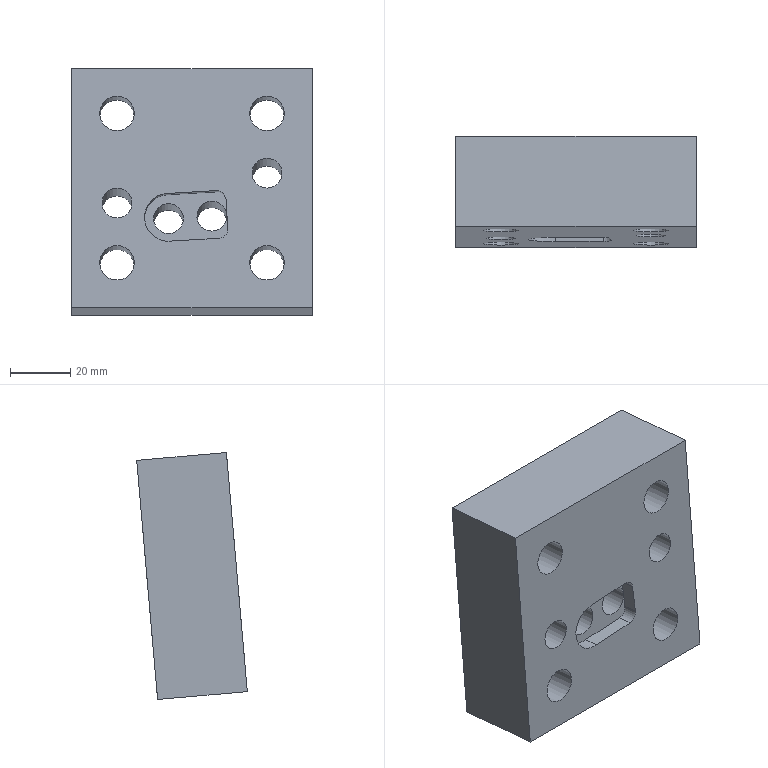Part | NX | features solid 2 | 1 solid | 29 faces | box 80 x 36.858 x 82.31 mm | volume 162259 mm3 | cylinder 15 | plane 14 | commonest cylinder face diameters 10 x4 11.5 x4 16.5 x4 6 x2 16 x1
STEP:
#1=CARTESIAN_POINT('',(-226.83,-137.19,-16.919));
#2=VERTEX_POINT('',#1);
#3=CARTESIAN_POINT('',(-242.835,-137.271,-17.849));
#4=VERTEX_POINT('',#3);
#5=CARTESIAN_POINT('',(-228.366,-137.198,-17.008));
#6=DIRECTION('',(0.9983,0.00508,0.05807));
#7=VECTOR('',#6,1000.);
#8=LINE('',#5,#7);
#9=EDGE_CURVE('',#2,#4,#8,.F.);
#10=ORIENTED_EDGE('',*,*,#9,.F.);
#11=CARTESIAN_POINT('',(-226.83,-142.171,-16.483));
#12=VERTEX_POINT('',#11);
#13=CARTESIAN_POINT('',(-226.83,-142.171,-16.483));
#14=DIRECTION('',(0.,0.9962,-0.08716));
#15=VECTOR('',#14,1000.);
#16=LINE('',#13,#15);
#17=EDGE_CURVE('',#2,#12,#16,.F.);
#18=ORIENTED_EDGE('',*,*,#17,.T.);
#19=CARTESIAN_POINT('',(-242.835,-142.252,-17.414));
#20=VERTEX_POINT('',#19);
#21=CARTESIAN_POINT('',(-192.383,-141.996,-14.479));
#22=DIRECTION('',(0.9983,0.00508,0.05807));
#23=VECTOR('',#22,1000.);
#24=LINE('',#21,#23);
#25=EDGE_CURVE('',#20,#12,#24,.T.);
#26=ORIENTED_EDGE('',*,*,#25,.F.);
#27=CARTESIAN_POINT('',(-242.835,-142.252,-17.414));
#28=DIRECTION('',(0.,0.9962,-0.08716));
#29=VECTOR('',#28,1000.);
#30=LINE('',#27,#29);
#31=EDGE_CURVE('',#20,#4,#30,.T.);
#32=ORIENTED_EDGE('',*,*,#31,.T.);
#33=EDGE_LOOP('',(#10,#18,#26,#32));
#34=FACE_BOUND('',#33,.T.);
#35=CARTESIAN_POINT('',(-228.366,-142.179,-16.572));
#36=DIRECTION('',(0.05829,-0.08701,-0.9945));
#37=DIRECTION('',(0.9983,0.00508,0.05807));
#38=AXIS2_PLACEMENT_3D('',#35,#36,#37);
#39=PLANE('',#38);
#40=ADVANCED_FACE('',(#34),#39,.T.);
#41=CARTESIAN_POINT('',(-260.,-140.42,3.528));
#42=VERTEX_POINT('',#41);
#43=CARTESIAN_POINT('',(-260.,-139.919,9.256));
#44=DIRECTION('',(0.,-0.9962,0.08716));
#45=DIRECTION('',(0.,-0.08716,-0.9962));
#46=AXIS2_PLACEMENT_3D('',#43,#44,#45);
#47=CIRCLE('',#46,5.75);
#48=EDGE_CURVE('',#42,#42,#47,.T.);
#49=ORIENTED_EDGE('',*,*,#48,.F.);
#50=EDGE_LOOP('',(#49));
#51=FACE_BOUND('',#50,.T.);
#52=CARTESIAN_POINT('',(-210.,-140.42,3.528));
#53=VERTEX_POINT('',#52);
#54=CARTESIAN_POINT('',(-210.,-139.919,9.256));
#55=DIRECTION('',(0.,-0.9962,0.08716));
#56=DIRECTION('',(0.,-0.08716,-0.9962));
#57=AXIS2_PLACEMENT_3D('',#54,#55,#56);
#58=CIRCLE('',#57,5.75);
#59=EDGE_CURVE('',#53,#53,#58,.F.);
#60=ORIENTED_EDGE('',*,*,#59,.T.);
#61=EDGE_LOOP('',(#60));
#62=FACE_BOUND('',#61,.T.);
#63=CARTESIAN_POINT('',(-210.,-142.098,-15.649));
#64=VERTEX_POINT('',#63);
#65=CARTESIAN_POINT('',(-210.,-141.662,-10.668));
#66=DIRECTION('',(0.,-0.9962,0.08716));
#67=DIRECTION('',(0.,-0.08716,-0.9962));
#68=AXIS2_PLACEMENT_3D('',#65,#66,#67);
#69=CIRCLE('',#68,5.);
#70=EDGE_CURVE('',#64,#64,#69,.F.);
#71=ORIENTED_EDGE('',*,*,#70,.T.);
#72=EDGE_LOOP('',(#71));
#73=FACE_BOUND('',#72,.T.);
#74=CARTESIAN_POINT('',(-195.,-138.612,24.199));
#75=VERTEX_POINT('',#74);
#76=CARTESIAN_POINT('',(-275.,-138.612,24.199));
#77=VERTEX_POINT('',#76);
#78=CARTESIAN_POINT('',(-195.,-138.612,24.199));
#79=DIRECTION('',(-1.,0.,0.));
#80=VECTOR('',#79,1000.);
#81=LINE('',#78,#80);
#82=EDGE_CURVE('',#75,#77,#81,.T.);
#83=ORIENTED_EDGE('',*,*,#82,.T.);
#84=CARTESIAN_POINT('',(-275.,-145.584,-55.497));
#85=VERTEX_POINT('',#84);
#86=CARTESIAN_POINT('',(-275.,-138.089,30.174));
#87=DIRECTION('',(0.,-0.08716,-0.9962));
#88=VECTOR('',#87,1000.);
#89=LINE('',#86,#88);
#90=EDGE_CURVE('',#85,#77,#89,.F.);
#91=ORIENTED_EDGE('',*,*,#90,.F.);
#92=CARTESIAN_POINT('',(-195.,-145.584,-55.497));
#93=VERTEX_POINT('',#92);
#94=CARTESIAN_POINT('',(-195.,-145.584,-55.497));
#95=DIRECTION('',(1.,0.,0.));
#96=VECTOR('',#95,1000.);
#97=LINE('',#94,#96);
#98=EDGE_CURVE('',#85,#93,#97,.T.);
#99=ORIENTED_EDGE('',*,*,#98,.T.);
#100=CARTESIAN_POINT('',(-195.,-142.665,-22.124));
#101=DIRECTION('',(0.,-0.08716,-0.9962));
#102=VECTOR('',#101,1000.);
#103=LINE('',#100,#102);
#104=EDGE_CURVE('',#75,#93,#103,.T.);
#105=ORIENTED_EDGE('',*,*,#104,.F.);
#106=EDGE_LOOP('',(#83,#91,#99,#105));
#107=FACE_BOUND('',#106,.T.);
#108=CARTESIAN_POINT('',(-260.,-142.97,-25.611));
#109=VERTEX_POINT('',#108);
#110=CARTESIAN_POINT('',(-260.,-142.534,-20.63));
#111=DIRECTION('',(0.,-0.9962,0.08716));
#112=DIRECTION('',(0.,-0.08716,-0.9962));
#113=AXIS2_PLACEMENT_3D('',#110,#111,#112);
#114=CIRCLE('',#113,5.);
#115=EDGE_CURVE('',#109,#109,#114,.F.);
#116=ORIENTED_EDGE('',*,*,#115,.T.);
#117=EDGE_LOOP('',(#116));
#118=FACE_BOUND('',#117,.T.);
#119=CARTESIAN_POINT('',(-260.,-144.778,-46.282));
#120=VERTEX_POINT('',#119);
#121=CARTESIAN_POINT('',(-260.,-144.277,-40.554));
#122=DIRECTION('',(0.,-0.9962,0.08716));
#123=DIRECTION('',(0.,-0.08716,-0.9962));
#124=AXIS2_PLACEMENT_3D('',#121,#122,#123);
#125=CIRCLE('',#124,5.75);
#126=EDGE_CURVE('',#120,#120,#125,.F.);
#127=ORIENTED_EDGE('',*,*,#126,.T.);
#128=EDGE_LOOP('',(#127));
#129=FACE_BOUND('',#128,.T.);
#130=CARTESIAN_POINT('',(-210.,-144.778,-46.282));
#131=VERTEX_POINT('',#130);
#132=CARTESIAN_POINT('',(-210.,-144.277,-40.554));
#133=DIRECTION('',(0.,-0.9962,0.08716));
#134=DIRECTION('',(0.,-0.08716,-0.9962));
#135=AXIS2_PLACEMENT_3D('',#132,#133,#134);
#136=CIRCLE('',#135,5.75);
#137=EDGE_CURVE('',#131,#131,#136,.T.);
#138=ORIENTED_EDGE('',*,*,#137,.F.);
#139=EDGE_LOOP('',(#138));
#140=FACE_BOUND('',#139,.T.);
#141=CARTESIAN_POINT('',(-241.904,-143.642,-33.299));
#142=VERTEX_POINT('',#141);
#143=CARTESIAN_POINT('',(-242.835,-142.95,-25.383));
#144=DIRECTION('',(0.,-0.9962,0.08716));
#145=DIRECTION('',(0.,-0.08716,-0.9962));
#146=AXIS2_PLACEMENT_3D('',#143,#144,#145);
#147=CIRCLE('',#146,8.);
#148=EDGE_CURVE('',#142,#20,#147,.F.);
#149=ORIENTED_EDGE('',*,*,#148,.T.);
#150=ORIENTED_EDGE('',*,*,#25,.T.);
#151=CARTESIAN_POINT('',(-223.66,-142.417,-19.295));
#152=VERTEX_POINT('',#151);
#153=CARTESIAN_POINT('',(-226.655,-142.432,-19.466));
#154=DIRECTION('',(0.,-0.9962,0.08716));
#155=DIRECTION('',(0.,-0.08716,-0.9962));
#156=AXIS2_PLACEMENT_3D('',#153,#154,#155);
#157=CIRCLE('',#156,3.);
#158=EDGE_CURVE('',#12,#152,#157,.F.);
#159=ORIENTED_EDGE('',*,*,#158,.T.);
#160=CARTESIAN_POINT('',(-223.09,-143.285,-29.214));
#161=VERTEX_POINT('',#160);
#162=CARTESIAN_POINT('',(-223.375,-142.851,-24.257));
#163=DIRECTION('',(0.05719,-0.08701,-0.9946));
#164=VECTOR('',#163,1000.);
#165=LINE('',#162,#164);
#166=EDGE_CURVE('',#152,#161,#165,.T.);
#167=ORIENTED_EDGE('',*,*,#166,.T.);
#168=CARTESIAN_POINT('',(-225.91,-143.561,-32.368));
#169=VERTEX_POINT('',#168);
#170=CARTESIAN_POINT('',(-226.085,-143.3,-29.385));
#171=DIRECTION('',(0.,-0.9962,0.08716));
#172=DIRECTION('',(0.,-0.08716,-0.9962));
#173=AXIS2_PLACEMENT_3D('',#170,#171,#172);
#174=CIRCLE('',#173,3.);
#175=EDGE_CURVE('',#161,#169,#174,.F.);
#176=ORIENTED_EDGE('',*,*,#175,.T.);
#177=CARTESIAN_POINT('',(-228.366,-143.573,-32.511));
#178=DIRECTION('',(-0.9983,-0.00508,-0.05807));
#179=VECTOR('',#178,1000.);
#180=LINE('',#177,#179);
#181=EDGE_CURVE('',#142,#169,#180,.F.);
#182=ORIENTED_EDGE('',*,*,#181,.F.);
#183=EDGE_LOOP('',(#149,#150,#159,#167,#176,#182));
#184=FACE_BOUND('',#183,.T.);
#185=CARTESIAN_POINT('',(-195.,-138.089,30.174));
#186=DIRECTION('',(0.,-0.9962,0.08716));
#187=DIRECTION('',(-1.,0.,0.));
#188=AXIS2_PLACEMENT_3D('',#185,#186,#187);
#189=PLANE('',#188);
#190=ADVANCED_FACE('',(#51,#62,#73,#107,#118,#129,#140,#184),#189,.T.);
#191=CARTESIAN_POINT('',(-260.,-124.257,16.167));
#192=VERTEX_POINT('',#191);
#193=CARTESIAN_POINT('',(-260.,-124.976,7.949));
#194=DIRECTION('',(0.,0.9962,-0.08716));
#195=DIRECTION('',(0.,0.08716,0.9962));
#196=AXIS2_PLACEMENT_3D('',#193,#194,#195);
#197=CIRCLE('',#196,8.25);
#198=EDGE_CURVE('',#192,#192,#197,.T.);
#199=ORIENTED_EDGE('',*,*,#198,.T.);
#200=EDGE_LOOP('',(#199));
#201=FACE_BOUND('',#200,.T.);
#202=CARTESIAN_POINT('',(-260.,-124.475,13.677));
#203=VERTEX_POINT('',#202);
#204=CARTESIAN_POINT('',(-260.,-124.976,7.949));
#205=DIRECTION('',(0.,0.9962,-0.08716));
#206=DIRECTION('',(0.,0.08716,0.9962));
#207=AXIS2_PLACEMENT_3D('',#204,#205,#206);
#208=CIRCLE('',#207,5.75);
#209=EDGE_CURVE('',#203,#203,#208,.F.);
#210=ORIENTED_EDGE('',*,*,#209,.T.);
#211=EDGE_LOOP('',(#210));
#212=FACE_BOUND('',#211,.T.);
#213=CARTESIAN_POINT('',(-260.,-124.976,7.949));
#214=DIRECTION('',(0.,0.9962,-0.08716));
#215=DIRECTION('',(-1.,0.,0.));
#216=AXIS2_PLACEMENT_3D('',#213,#214,#215);
#217=PLANE('',#216);
#218=ADVANCED_FACE('',(#201,#212),#217,.T.);
#219=CARTESIAN_POINT('',(-210.,-128.615,-33.643));
#220=VERTEX_POINT('',#219);
#221=CARTESIAN_POINT('',(-210.,-129.334,-41.861));
#222=DIRECTION('',(0.,0.9962,-0.08716));
#223=DIRECTION('',(0.,0.08716,0.9962));
#224=AXIS2_PLACEMENT_3D('',#221,#222,#223);
#225=CIRCLE('',#224,8.25);
#226=EDGE_CURVE('',#220,#220,#225,.T.);
#227=ORIENTED_EDGE('',*,*,#226,.T.);
#228=EDGE_LOOP('',(#227));
#229=FACE_BOUND('',#228,.T.);
#230=CARTESIAN_POINT('',(-210.,-128.833,-36.133));
#231=VERTEX_POINT('',#230);
#232=CARTESIAN_POINT('',(-210.,-129.334,-41.861));
#233=DIRECTION('',(0.,0.9962,-0.08716));
#234=DIRECTION('',(0.,0.08716,0.9962));
#235=AXIS2_PLACEMENT_3D('',#232,#233,#234);
#236=CIRCLE('',#235,5.75);
#237=EDGE_CURVE('',#231,#231,#236,.F.);
#238=ORIENTED_EDGE('',*,*,#237,.T.);
#239=EDGE_LOOP('',(#238));
#240=FACE_BOUND('',#239,.T.);
#241=CARTESIAN_POINT('',(-210.,-129.334,-41.861));
#242=DIRECTION('',(0.,0.9962,-0.08716));
#243=DIRECTION('',(-1.,0.,0.));
#244=AXIS2_PLACEMENT_3D('',#241,#242,#243);
#245=PLANE('',#244);
#246=ADVANCED_FACE('',(#229,#240),#245,.T.);
#247=CARTESIAN_POINT('',(-228.366,-113.426,-32.137));
#248=VERTEX_POINT('',#247);
#249=CARTESIAN_POINT('',(-228.366,-112.99,-27.156));
#250=DIRECTION('',(0.,-0.9962,0.08716));
#251=DIRECTION('',(0.,-0.08716,-0.9962));
#252=AXIS2_PLACEMENT_3D('',#249,#250,#251);
#253=CIRCLE('',#252,5.);
#254=EDGE_CURVE('',#248,#248,#253,.F.);
#255=ORIENTED_EDGE('',*,*,#254,.F.);
#256=EDGE_LOOP('',(#255));
#257=FACE_BOUND('',#256,.T.);
#258=CARTESIAN_POINT('',(-242.835,-113.5,-32.979));
#259=VERTEX_POINT('',#258);
#260=CARTESIAN_POINT('',(-242.835,-113.064,-27.998));
#261=DIRECTION('',(0.,-0.9962,0.08716));
#262=DIRECTION('',(0.,-0.08716,-0.9962));
#263=AXIS2_PLACEMENT_3D('',#260,#261,#262);
#264=CIRCLE('',#263,5.);
#265=EDGE_CURVE('',#259,#259,#264,.F.);
#266=ORIENTED_EDGE('',*,*,#265,.F.);
#267=EDGE_LOOP('',(#266));
#268=FACE_BOUND('',#267,.T.);
#269=CARTESIAN_POINT('',(-210.,-112.212,-18.264));
#270=VERTEX_POINT('',#269);
#271=CARTESIAN_POINT('',(-210.,-111.776,-13.283));
#272=DIRECTION('',(0.,-0.9962,0.08716));
#273=DIRECTION('',(0.,-0.08716,-0.9962));
#274=AXIS2_PLACEMENT_3D('',#271,#272,#273);
#275=CIRCLE('',#274,5.);
#276=EDGE_CURVE('',#270,#270,#275,.T.);
#277=ORIENTED_EDGE('',*,*,#276,.T.);
#278=EDGE_LOOP('',(#277));
#279=FACE_BOUND('',#278,.T.);
#280=CARTESIAN_POINT('',(-260.,-113.084,-28.226));
#281=VERTEX_POINT('',#280);
#282=CARTESIAN_POINT('',(-260.,-112.648,-23.245));
#283=DIRECTION('',(0.,-0.9962,0.08716));
#284=DIRECTION('',(0.,-0.08716,-0.9962));
#285=AXIS2_PLACEMENT_3D('',#282,#283,#284);
#286=CIRCLE('',#285,5.);
#287=EDGE_CURVE('',#281,#281,#286,.T.);
#288=ORIENTED_EDGE('',*,*,#287,.T.);
#289=EDGE_LOOP('',(#288));
#290=FACE_BOUND('',#289,.T.);
#291=CARTESIAN_POINT('',(-260.,-110.752,-1.577));
#292=VERTEX_POINT('',#291);
#293=CARTESIAN_POINT('',(-260.,-110.033,6.641));
#294=DIRECTION('',(0.,-0.9962,0.08716));
#295=DIRECTION('',(0.,-0.08716,-0.9962));
#296=AXIS2_PLACEMENT_3D('',#293,#294,#295);
#297=CIRCLE('',#296,8.25);
#298=EDGE_CURVE('',#292,#292,#297,.F.);
#299=ORIENTED_EDGE('',*,*,#298,.F.);
#300=EDGE_LOOP('',(#299));
#301=FACE_BOUND('',#300,.T.);
#302=CARTESIAN_POINT('',(-260.,-115.11,-51.387));
#303=VERTEX_POINT('',#302);
#304=CARTESIAN_POINT('',(-260.,-114.391,-43.169));
#305=DIRECTION('',(0.,-0.9962,0.08716));
#306=DIRECTION('',(0.,-0.08716,-0.9962));
#307=AXIS2_PLACEMENT_3D('',#304,#305,#306);
#308=CIRCLE('',#307,8.25);
#309=EDGE_CURVE('',#303,#303,#308,.T.);
#310=ORIENTED_EDGE('',*,*,#309,.T.);
#311=EDGE_LOOP('',(#310));
#312=FACE_BOUND('',#311,.T.);
#313=CARTESIAN_POINT('',(-195.,-108.726,21.584));
#314=VERTEX_POINT('',#313);
#315=CARTESIAN_POINT('',(-275.,-108.726,21.584));
#316=VERTEX_POINT('',#315);
#317=CARTESIAN_POINT('',(-195.,-108.726,21.584));
#318=DIRECTION('',(1.,0.,0.));
#319=VECTOR('',#318,1000.);
#320=LINE('',#317,#319);
#321=EDGE_CURVE('',#314,#316,#320,.F.);
#322=ORIENTED_EDGE('',*,*,#321,.F.);
#323=CARTESIAN_POINT('',(-195.,-115.698,-58.111));
#324=VERTEX_POINT('',#323);
#325=CARTESIAN_POINT('',(-195.,-108.203,27.56));
#326=DIRECTION('',(0.,0.08716,0.9962));
#327=VECTOR('',#326,1000.);
#328=LINE('',#325,#327);
#329=EDGE_CURVE('',#314,#324,#328,.F.);
#330=ORIENTED_EDGE('',*,*,#329,.T.);
#331=CARTESIAN_POINT('',(-275.,-115.698,-58.111));
#332=VERTEX_POINT('',#331);
#333=CARTESIAN_POINT('',(-195.,-115.698,-58.111));
#334=DIRECTION('',(-1.,0.,0.));
#335=VECTOR('',#334,1000.);
#336=LINE('',#333,#335);
#337=EDGE_CURVE('',#332,#324,#336,.F.);
#338=ORIENTED_EDGE('',*,*,#337,.F.);
#339=CARTESIAN_POINT('',(-275.,-108.203,27.56));
#340=DIRECTION('',(0.,-0.08716,-0.9962));
#341=VECTOR('',#340,1000.);
#342=LINE('',#339,#341);
#343=EDGE_CURVE('',#332,#316,#342,.F.);
#344=ORIENTED_EDGE('',*,*,#343,.T.);
#345=EDGE_LOOP('',(#322,#330,#338,#344));
#346=FACE_BOUND('',#345,.T.);
#347=CARTESIAN_POINT('',(-210.,-110.752,-1.577));
#348=VERTEX_POINT('',#347);
#349=CARTESIAN_POINT('',(-210.,-110.033,6.641));
#350=DIRECTION('',(0.,-0.9962,0.08716));
#351=DIRECTION('',(0.,-0.08716,-0.9962));
#352=AXIS2_PLACEMENT_3D('',#349,#350,#351);
#353=CIRCLE('',#352,8.25);
#354=EDGE_CURVE('',#348,#348,#353,.T.);
#355=ORIENTED_EDGE('',*,*,#354,.T.);
#356=EDGE_LOOP('',(#355));
#357=FACE_BOUND('',#356,.T.);
#358=CARTESIAN_POINT('',(-210.,-115.11,-51.387));
#359=VERTEX_POINT('',#358);
#360=CARTESIAN_POINT('',(-210.,-114.391,-43.169));
#361=DIRECTION('',(0.,-0.9962,0.08716));
#362=DIRECTION('',(0.,-0.08716,-0.9962));
#363=AXIS2_PLACEMENT_3D('',#360,#361,#362);
#364=CIRCLE('',#363,8.25);
#365=EDGE_CURVE('',#359,#359,#364,.F.);
#366=ORIENTED_EDGE('',*,*,#365,.F.);
#367=EDGE_LOOP('',(#366));
#368=FACE_BOUND('',#367,.T.);
#369=CARTESIAN_POINT('',(-195.,-108.203,27.56));
#370=DIRECTION('',(0.,-0.9962,0.08716));
#371=DIRECTION('',(-1.,0.,0.));
#372=AXIS2_PLACEMENT_3D('',#369,#370,#371);
#373=PLANE('',#372);
#374=ADVANCED_FACE('',(#257,#268,#279,#290,#301,#312,#346,#357,#368),#373,.F.);
#375=ORIENTED_EDGE('',*,*,#321,.T.);
#376=CARTESIAN_POINT('',(-275.,-138.612,24.199));
#377=DIRECTION('',(0.,0.9962,-0.08716));
#378=VECTOR('',#377,1000.);
#379=LINE('',#376,#378);
#380=EDGE_CURVE('',#77,#316,#379,.T.);
#381=ORIENTED_EDGE('',*,*,#380,.F.);
#382=ORIENTED_EDGE('',*,*,#82,.F.);
#383=CARTESIAN_POINT('',(-195.,-138.612,24.199));
#384=DIRECTION('',(0.,0.9962,-0.08716));
#385=VECTOR('',#384,1000.);
#386=LINE('',#383,#385);
#387=EDGE_CURVE('',#75,#314,#386,.T.);
#388=ORIENTED_EDGE('',*,*,#387,.T.);
#389=EDGE_LOOP('',(#375,#381,#382,#388));
#390=FACE_BOUND('',#389,.T.);
#391=CARTESIAN_POINT('',(-195.,-138.612,24.199));
#392=DIRECTION('',(0.,-0.08716,-0.9962));
#393=DIRECTION('',(0.,0.9962,-0.08716));
#394=AXIS2_PLACEMENT_3D('',#391,#392,#393);
#395=PLANE('',#394);
#396=ADVANCED_FACE('',(#390),#395,.F.);
#397=ORIENTED_EDGE('',*,*,#329,.F.);
#398=ORIENTED_EDGE('',*,*,#387,.F.);
#399=ORIENTED_EDGE('',*,*,#104,.T.);
#400=CARTESIAN_POINT('',(-195.,-145.584,-55.497));
#401=DIRECTION('',(0.,-0.9962,0.08716));
#402=VECTOR('',#401,1000.);
#403=LINE('',#400,#402);
#404=EDGE_CURVE('',#93,#324,#403,.F.);
#405=ORIENTED_EDGE('',*,*,#404,.T.);
#406=EDGE_LOOP('',(#397,#398,#399,#405));
#407=FACE_BOUND('',#406,.T.);
#408=CARTESIAN_POINT('',(-195.,-142.665,-22.124));
#409=DIRECTION('',(1.,0.,0.));
#410=DIRECTION('',(0.,0.,-1.));
#411=AXIS2_PLACEMENT_3D('',#408,#409,#410);
#412=PLANE('',#411);
#413=ADVANCED_FACE('',(#407),#412,.T.);
#414=ORIENTED_EDGE('',*,*,#337,.T.);
#415=ORIENTED_EDGE('',*,*,#404,.F.);
#416=ORIENTED_EDGE('',*,*,#98,.F.);
#417=CARTESIAN_POINT('',(-275.,-145.584,-55.497));
#418=DIRECTION('',(0.,0.9962,-0.08716));
#419=VECTOR('',#418,1000.);
#420=LINE('',#417,#419);
#421=EDGE_CURVE('',#85,#332,#420,.T.);
#422=ORIENTED_EDGE('',*,*,#421,.T.);
#423=EDGE_LOOP('',(#414,#415,#416,#422));
#424=FACE_BOUND('',#423,.T.);
#425=CARTESIAN_POINT('',(-195.,-145.584,-55.497));
#426=DIRECTION('',(0.,-0.08716,-0.9962));
#427=DIRECTION('',(0.,0.9962,-0.08716));
#428=AXIS2_PLACEMENT_3D('',#425,#426,#427);
#429=PLANE('',#428);
#430=ADVANCED_FACE('',(#424),#429,.T.);
#431=ORIENTED_EDGE('',*,*,#343,.F.);
#432=ORIENTED_EDGE('',*,*,#421,.F.);
#433=ORIENTED_EDGE('',*,*,#90,.T.);
#434=ORIENTED_EDGE('',*,*,#380,.T.);
#435=EDGE_LOOP('',(#431,#432,#433,#434));
#436=FACE_BOUND('',#435,.T.);
#437=CARTESIAN_POINT('',(-275.,-138.089,30.174));
#438=DIRECTION('',(-1.,0.,0.));
#439=DIRECTION('',(0.,0.,1.));
#440=AXIS2_PLACEMENT_3D('',#437,#438,#439);
#441=PLANE('',#440);
#442=ADVANCED_FACE('',(#436),#441,.T.);
#443=ORIENTED_EDGE('',*,*,#309,.F.);
#444=EDGE_LOOP('',(#443));
#445=FACE_BOUND('',#444,.T.);
#446=CARTESIAN_POINT('',(-260.,-130.053,-50.08));
#447=VERTEX_POINT('',#446);
#448=CARTESIAN_POINT('',(-260.,-129.334,-41.861));
#449=DIRECTION('',(0.,-0.9962,0.08716));
#450=DIRECTION('',(0.,-0.08716,-0.9962));
#451=AXIS2_PLACEMENT_3D('',#448,#449,#450);
#452=CIRCLE('',#451,8.25);
#453=EDGE_CURVE('',#447,#447,#452,.T.);
#454=ORIENTED_EDGE('',*,*,#453,.T.);
#455=EDGE_LOOP('',(#454));
#456=FACE_BOUND('',#455,.T.);
#457=CARTESIAN_POINT('',(-260.,-119.372,-42.733));
#458=DIRECTION('',(0.,-0.9962,0.08716));
#459=DIRECTION('',(1.,0.,0.));
#460=AXIS2_PLACEMENT_3D('',#457,#458,#459);
#461=CYLINDRICAL_SURFACE('',#460,8.25);
#462=ADVANCED_FACE('',(#445,#456),#461,.F.);
#463=CARTESIAN_POINT('',(-260.,-129.835,-47.589));
#464=VERTEX_POINT('',#463);
#465=CARTESIAN_POINT('',(-260.,-129.334,-41.861));
#466=DIRECTION('',(0.,-0.9962,0.08716));
#467=DIRECTION('',(0.,-0.08716,-0.9962));
#468=AXIS2_PLACEMENT_3D('',#465,#466,#467);
#469=CIRCLE('',#468,5.75);
#470=EDGE_CURVE('',#464,#464,#469,.T.);
#471=ORIENTED_EDGE('',*,*,#470,.T.);
#472=EDGE_LOOP('',(#471));
#473=FACE_BOUND('',#472,.T.);
#474=ORIENTED_EDGE('',*,*,#453,.F.);
#475=EDGE_LOOP('',(#474));
#476=FACE_BOUND('',#475,.T.);
#477=CARTESIAN_POINT('',(-260.,-129.334,-41.861));
#478=DIRECTION('',(0.,-0.9962,0.08716));
#479=DIRECTION('',(1.,0.,0.));
#480=AXIS2_PLACEMENT_3D('',#477,#478,#479);
#481=PLANE('',#480);
#482=ADVANCED_FACE('',(#473,#476),#481,.F.);
#483=ORIENTED_EDGE('',*,*,#298,.T.);
#484=EDGE_LOOP('',(#483));
#485=FACE_BOUND('',#484,.T.);
#486=ORIENTED_EDGE('',*,*,#198,.F.);
#487=EDGE_LOOP('',(#486));
#488=FACE_BOUND('',#487,.T.);
#489=CARTESIAN_POINT('',(-260.,-115.014,7.077));
#490=DIRECTION('',(0.,-0.9962,0.08716));
#491=DIRECTION('',(1.,0.,0.));
#492=AXIS2_PLACEMENT_3D('',#489,#490,#491);
#493=CYLINDRICAL_SURFACE('',#492,8.25);
#494=ADVANCED_FACE('',(#485,#488),#493,.F.);
#495=ORIENTED_EDGE('',*,*,#354,.F.);
#496=EDGE_LOOP('',(#495));
#497=FACE_BOUND('',#496,.T.);
#498=CARTESIAN_POINT('',(-210.,-125.695,-0.2701));
#499=VERTEX_POINT('',#498);
#500=CARTESIAN_POINT('',(-210.,-124.976,7.949));
#501=DIRECTION('',(0.,-0.9962,0.08716));
#502=DIRECTION('',(0.,-0.08716,-0.9962));
#503=AXIS2_PLACEMENT_3D('',#500,#501,#502);
#504=CIRCLE('',#503,8.25);
#505=EDGE_CURVE('',#499,#499,#504,.T.);
#506=ORIENTED_EDGE('',*,*,#505,.T.);
#507=EDGE_LOOP('',(#506));
#508=FACE_BOUND('',#507,.T.);
#509=CARTESIAN_POINT('',(-210.,-115.014,7.077));
#510=DIRECTION('',(0.,-0.9962,0.08716));
#511=DIRECTION('',(1.,0.,0.));
#512=AXIS2_PLACEMENT_3D('',#509,#510,#511);
#513=CYLINDRICAL_SURFACE('',#512,8.25);
#514=ADVANCED_FACE('',(#497,#508),#513,.F.);
#515=CARTESIAN_POINT('',(-210.,-125.477,2.22));
#516=VERTEX_POINT('',#515);
#517=CARTESIAN_POINT('',(-210.,-124.976,7.949));
#518=DIRECTION('',(0.,-0.9962,0.08716));
#519=DIRECTION('',(0.,-0.08716,-0.9962));
#520=AXIS2_PLACEMENT_3D('',#517,#518,#519);
#521=CIRCLE('',#520,5.75);
#522=EDGE_CURVE('',#516,#516,#521,.T.);
#523=ORIENTED_EDGE('',*,*,#522,.T.);
#524=EDGE_LOOP('',(#523));
#525=FACE_BOUND('',#524,.T.);
#526=ORIENTED_EDGE('',*,*,#505,.F.);
#527=EDGE_LOOP('',(#526));
#528=FACE_BOUND('',#527,.T.);
#529=CARTESIAN_POINT('',(-210.,-124.976,7.949));
#530=DIRECTION('',(0.,-0.9962,0.08716));
#531=DIRECTION('',(1.,0.,0.));
#532=AXIS2_PLACEMENT_3D('',#529,#530,#531);
#533=PLANE('',#532);
#534=ADVANCED_FACE('',(#525,#528),#533,.F.);
#535=ORIENTED_EDGE('',*,*,#365,.T.);
#536=EDGE_LOOP('',(#535));
#537=FACE_BOUND('',#536,.T.);
#538=ORIENTED_EDGE('',*,*,#226,.F.);
#539=EDGE_LOOP('',(#538));
#540=FACE_BOUND('',#539,.T.);
#541=CARTESIAN_POINT('',(-210.,-119.372,-42.733));
#542=DIRECTION('',(0.,-0.9962,0.08716));
#543=DIRECTION('',(1.,0.,0.));
#544=AXIS2_PLACEMENT_3D('',#541,#542,#543);
#545=CYLINDRICAL_SURFACE('',#544,8.25);
#546=ADVANCED_FACE('',(#537,#540),#545,.F.);
#547=ORIENTED_EDGE('',*,*,#287,.F.);
#548=EDGE_LOOP('',(#547));
#549=FACE_BOUND('',#548,.T.);
#550=ORIENTED_EDGE('',*,*,#115,.F.);
#551=EDGE_LOOP('',(#550));
#552=FACE_BOUND('',#551,.T.);
#553=CARTESIAN_POINT('',(-260.,-117.629,-22.809));
#554=DIRECTION('',(0.,-0.9962,0.08716));
#555=DIRECTION('',(1.,0.,0.));
#556=AXIS2_PLACEMENT_3D('',#553,#554,#555);
#557=CYLINDRICAL_SURFACE('',#556,5.);
#558=ADVANCED_FACE('',(#549,#552),#557,.F.);
#559=ORIENTED_EDGE('',*,*,#470,.F.);
#560=EDGE_LOOP('',(#559));
#561=FACE_BOUND('',#560,.T.);
#562=ORIENTED_EDGE('',*,*,#126,.F.);
#563=EDGE_LOOP('',(#562));
#564=FACE_BOUND('',#563,.T.);
#565=CARTESIAN_POINT('',(-260.,-119.372,-42.733));
#566=DIRECTION('',(0.,-0.9962,0.08716));
#567=DIRECTION('',(1.,0.,0.));
#568=AXIS2_PLACEMENT_3D('',#565,#566,#567);
#569=CYLINDRICAL_SURFACE('',#568,5.75);
#570=ADVANCED_FACE('',(#561,#564),#569,.F.);
#571=ORIENTED_EDGE('',*,*,#237,.F.);
#572=EDGE_LOOP('',(#571));
#573=FACE_BOUND('',#572,.T.);
#574=ORIENTED_EDGE('',*,*,#137,.T.);
#575=EDGE_LOOP('',(#574));
#576=FACE_BOUND('',#575,.T.);
#577=CARTESIAN_POINT('',(-210.,-119.372,-42.733));
#578=DIRECTION('',(0.,-0.9962,0.08716));
#579=DIRECTION('',(1.,0.,0.));
#580=AXIS2_PLACEMENT_3D('',#577,#578,#579);
#581=CYLINDRICAL_SURFACE('',#580,5.75);
#582=ADVANCED_FACE('',(#573,#576),#581,.F.);
#583=ORIENTED_EDGE('',*,*,#276,.F.);
#584=EDGE_LOOP('',(#583));
#585=FACE_BOUND('',#584,.T.);
#586=ORIENTED_EDGE('',*,*,#70,.F.);
#587=EDGE_LOOP('',(#586));
#588=FACE_BOUND('',#587,.T.);
#589=CARTESIAN_POINT('',(-210.,-116.757,-12.847));
#590=DIRECTION('',(0.,-0.9962,0.08716));
#591=DIRECTION('',(1.,0.,0.));
#592=AXIS2_PLACEMENT_3D('',#589,#590,#591);
#593=CYLINDRICAL_SURFACE('',#592,5.);
#594=ADVANCED_FACE('',(#585,#588),#593,.F.);
#595=ORIENTED_EDGE('',*,*,#522,.F.);
#596=EDGE_LOOP('',(#595));
#597=FACE_BOUND('',#596,.T.);
#598=ORIENTED_EDGE('',*,*,#59,.F.);
#599=EDGE_LOOP('',(#598));
#600=FACE_BOUND('',#599,.T.);
#601=CARTESIAN_POINT('',(-210.,-115.014,7.077));
#602=DIRECTION('',(0.,-0.9962,0.08716));
#603=DIRECTION('',(1.,0.,0.));
#604=AXIS2_PLACEMENT_3D('',#601,#602,#603);
#605=CYLINDRICAL_SURFACE('',#604,5.75);
#606=ADVANCED_FACE('',(#597,#600),#605,.F.);
#607=ORIENTED_EDGE('',*,*,#209,.F.);
#608=EDGE_LOOP('',(#607));
#609=FACE_BOUND('',#608,.T.);
#610=ORIENTED_EDGE('',*,*,#48,.T.);
#611=EDGE_LOOP('',(#610));
#612=FACE_BOUND('',#611,.T.);
#613=CARTESIAN_POINT('',(-260.,-115.014,7.077));
#614=DIRECTION('',(0.,-0.9962,0.08716));
#615=DIRECTION('',(1.,0.,0.));
#616=AXIS2_PLACEMENT_3D('',#613,#614,#615);
#617=CYLINDRICAL_SURFACE('',#616,5.75);
#618=ADVANCED_FACE('',(#609,#612),#617,.F.);
#619=ORIENTED_EDGE('',*,*,#265,.T.);
#620=EDGE_LOOP('',(#619));
#621=FACE_BOUND('',#620,.T.);
#622=CARTESIAN_POINT('',(-242.835,-137.533,-20.838));
#623=VERTEX_POINT('',#622);
#624=CARTESIAN_POINT('',(-242.835,-137.969,-25.819));
#625=DIRECTION('',(0.,0.9962,-0.08716));
#626=DIRECTION('',(0.,0.08716,0.9962));
#627=AXIS2_PLACEMENT_3D('',#624,#625,#626);
#628=CIRCLE('',#627,5.);
#629=EDGE_CURVE('',#623,#623,#628,.F.);
#630=ORIENTED_EDGE('',*,*,#629,.T.);
#631=EDGE_LOOP('',(#630));
#632=FACE_BOUND('',#631,.T.);
#633=CARTESIAN_POINT('',(-242.835,-71.409,-31.642));
#634=DIRECTION('',(0.,-0.9962,0.08716));
#635=DIRECTION('',(0.,-0.08716,-0.9962));
#636=AXIS2_PLACEMENT_3D('',#633,#634,#635);
#637=CYLINDRICAL_SURFACE('',#636,5.);
#638=ADVANCED_FACE('',(#621,#632),#637,.F.);
#639=CARTESIAN_POINT('',(-223.375,-137.87,-24.693));
#640=VERTEX_POINT('',#639);
#641=CARTESIAN_POINT('',(-223.66,-137.436,-19.731));
#642=VERTEX_POINT('',#641);
#643=CARTESIAN_POINT('',(-223.375,-137.87,-24.693));
#644=DIRECTION('',(-0.05719,0.08701,0.9946));
#645=VECTOR('',#644,1000.);
#646=LINE('',#643,#645);
#647=EDGE_CURVE('',#640,#642,#646,.T.);
#648=ORIENTED_EDGE('',*,*,#647,.T.);
#649=CARTESIAN_POINT('',(-226.655,-137.451,-19.902));
#650=DIRECTION('',(0.,0.9962,-0.08716));
#651=DIRECTION('',(-1.,0.,0.));
#652=AXIS2_PLACEMENT_3D('',#649,#650,#651);
#653=CIRCLE('',#652,3.);
#654=EDGE_CURVE('',#642,#2,#653,.F.);
#655=ORIENTED_EDGE('',*,*,#654,.T.);
#656=ORIENTED_EDGE('',*,*,#9,.T.);
#657=CARTESIAN_POINT('',(-241.904,-138.661,-33.734));
#658=VERTEX_POINT('',#657);
#659=CARTESIAN_POINT('',(-242.835,-137.969,-25.819));
#660=DIRECTION('',(0.,0.9962,-0.08716));
#661=DIRECTION('',(-1.,0.,0.));
#662=AXIS2_PLACEMENT_3D('',#659,#660,#661);
#663=CIRCLE('',#662,8.);
#664=EDGE_CURVE('',#4,#658,#663,.F.);
#665=ORIENTED_EDGE('',*,*,#664,.T.);
#666=CARTESIAN_POINT('',(-225.91,-138.58,-32.804));
#667=VERTEX_POINT('',#666);
#668=CARTESIAN_POINT('',(-228.366,-138.592,-32.947));
#669=DIRECTION('',(0.9983,0.00508,0.05807));
#670=VECTOR('',#669,1000.);
#671=LINE('',#668,#670);
#672=EDGE_CURVE('',#658,#667,#671,.T.);
#673=ORIENTED_EDGE('',*,*,#672,.T.);
#674=CARTESIAN_POINT('',(-223.09,-138.304,-29.65));
#675=VERTEX_POINT('',#674);
#676=CARTESIAN_POINT('',(-226.085,-138.319,-29.821));
#677=DIRECTION('',(0.,0.9962,-0.08716));
#678=DIRECTION('',(-1.,0.,0.));
#679=AXIS2_PLACEMENT_3D('',#676,#677,#678);
#680=CIRCLE('',#679,3.);
#681=EDGE_CURVE('',#667,#675,#680,.F.);
#682=ORIENTED_EDGE('',*,*,#681,.T.);
#683=CARTESIAN_POINT('',(-223.375,-137.87,-24.693));
#684=DIRECTION('',(-0.05719,0.08701,0.9946));
#685=VECTOR('',#684,1000.);
#686=LINE('',#683,#685);
#687=EDGE_CURVE('',#675,#640,#686,.T.);
#688=ORIENTED_EDGE('',*,*,#687,.T.);
#689=CARTESIAN_POINT('',(-228.366,-137.895,-24.977));
#690=DIRECTION('',(0.,-0.9962,0.08716));
#691=DIRECTION('',(0.,-0.08716,-0.9962));
#692=AXIS2_PLACEMENT_3D('',#689,#690,#691);
#693=CIRCLE('',#692,5.);
#694=EDGE_CURVE('',#640,#640,#693,.F.);
#695=ORIENTED_EDGE('',*,*,#694,.T.);
#696=EDGE_LOOP('',(#648,#655,#656,#665,#673,#682,#688,#695));
#697=FACE_BOUND('',#696,.T.);
#698=ORIENTED_EDGE('',*,*,#629,.F.);
#699=EDGE_LOOP('',(#698));
#700=FACE_BOUND('',#699,.T.);
#701=CARTESIAN_POINT('',(-242.835,-137.969,-25.819));
#702=DIRECTION('',(0.,0.9962,-0.08716));
#703=DIRECTION('',(0.,0.08716,0.9962));
#704=AXIS2_PLACEMENT_3D('',#701,#702,#703);
#705=PLANE('',#704);
#706=ADVANCED_FACE('',(#697,#700),#705,.F.);
#707=ORIENTED_EDGE('',*,*,#148,.F.);
#708=CARTESIAN_POINT('',(-241.904,-128.699,-34.606));
#709=DIRECTION('',(0.,-0.9962,0.08716));
#710=VECTOR('',#709,1000.);
#711=LINE('',#708,#710);
#712=EDGE_CURVE('',#142,#658,#711,.F.);
#713=ORIENTED_EDGE('',*,*,#712,.T.);
#714=ORIENTED_EDGE('',*,*,#664,.F.);
#715=ORIENTED_EDGE('',*,*,#31,.F.);
#716=EDGE_LOOP('',(#707,#713,#714,#715));
#717=FACE_BOUND('',#716,.T.);
#718=CARTESIAN_POINT('',(-242.835,-128.007,-26.691));
#719=DIRECTION('',(0.,-0.9962,0.08716));
#720=DIRECTION('',(0.,-0.08716,-0.9962));
#721=AXIS2_PLACEMENT_3D('',#718,#719,#720);
#722=CYLINDRICAL_SURFACE('',#721,8.);
#723=ADVANCED_FACE('',(#717),#722,.F.);
#724=ORIENTED_EDGE('',*,*,#254,.T.);
#725=EDGE_LOOP('',(#724));
#726=FACE_BOUND('',#725,.T.);
#727=ORIENTED_EDGE('',*,*,#694,.F.);
#728=EDGE_LOOP('',(#727));
#729=FACE_BOUND('',#728,.T.);
#730=CARTESIAN_POINT('',(-228.366,-71.336,-30.801));
#731=DIRECTION('',(0.,-0.9962,0.08716));
#732=DIRECTION('',(0.,-0.08716,-0.9962));
#733=AXIS2_PLACEMENT_3D('',#730,#731,#732);
#734=CYLINDRICAL_SURFACE('',#733,5.);
#735=ADVANCED_FACE('',(#726,#729),#734,.F.);
#736=ORIENTED_EDGE('',*,*,#166,.F.);
#737=CARTESIAN_POINT('',(-223.66,-126.478,-20.69));
#738=DIRECTION('',(0.,-0.9962,0.08716));
#739=VECTOR('',#738,1000.);
#740=LINE('',#737,#739);
#741=EDGE_CURVE('',#152,#642,#740,.F.);
#742=ORIENTED_EDGE('',*,*,#741,.T.);
#743=ORIENTED_EDGE('',*,*,#647,.F.);
#744=ORIENTED_EDGE('',*,*,#687,.F.);
#745=CARTESIAN_POINT('',(-223.09,-127.346,-30.608));
#746=DIRECTION('',(0.,0.9962,-0.08716));
#747=VECTOR('',#746,1000.);
#748=LINE('',#745,#747);
#749=EDGE_CURVE('',#675,#161,#748,.F.);
#750=ORIENTED_EDGE('',*,*,#749,.T.);
#751=EDGE_LOOP('',(#736,#742,#743,#744,#750));
#752=FACE_BOUND('',#751,.T.);
#753=CARTESIAN_POINT('',(-223.317,-126.999,-26.646));
#754=DIRECTION('',(-0.9984,-0.004985,-0.05697));
#755=DIRECTION('',(0.,-0.9962,0.08716));
#756=AXIS2_PLACEMENT_3D('',#753,#754,#755);
#757=PLANE('',#756);
#758=ADVANCED_FACE('',(#752),#757,.T.);
#759=ORIENTED_EDGE('',*,*,#181,.T.);
#760=CARTESIAN_POINT('',(-225.91,-143.561,-32.368));
#761=DIRECTION('',(0.,0.9962,-0.08716));
#762=VECTOR('',#761,1000.);
#763=LINE('',#760,#762);
#764=EDGE_CURVE('',#169,#667,#763,.T.);
#765=ORIENTED_EDGE('',*,*,#764,.T.);
#766=ORIENTED_EDGE('',*,*,#672,.F.);
#767=ORIENTED_EDGE('',*,*,#712,.F.);
#768=EDGE_LOOP('',(#759,#765,#766,#767));
#769=FACE_BOUND('',#768,.T.);
#770=CARTESIAN_POINT('',(-228.366,-143.573,-32.511));
#771=DIRECTION('',(0.05829,-0.08701,-0.9945));
#772=DIRECTION('',(0.9983,0.00508,0.05807));
#773=AXIS2_PLACEMENT_3D('',#770,#771,#772);
#774=PLANE('',#773);
#775=ADVANCED_FACE('',(#769),#774,.F.);
#776=ORIENTED_EDGE('',*,*,#158,.F.);
#777=ORIENTED_EDGE('',*,*,#17,.F.);
#778=ORIENTED_EDGE('',*,*,#654,.F.);
#779=ORIENTED_EDGE('',*,*,#741,.F.);
#780=EDGE_LOOP('',(#776,#777,#778,#779));
#781=FACE_BOUND('',#780,.T.);
#782=CARTESIAN_POINT('',(-226.655,-126.493,-20.861));
#783=DIRECTION('',(0.,-0.9962,0.08716));
#784=DIRECTION('',(1.,0.,0.));
#785=AXIS2_PLACEMENT_3D('',#782,#783,#784);
#786=CYLINDRICAL_SURFACE('',#785,3.);
#787=ADVANCED_FACE('',(#781),#786,.F.);
#788=ORIENTED_EDGE('',*,*,#175,.F.);
#789=ORIENTED_EDGE('',*,*,#749,.F.);
#790=ORIENTED_EDGE('',*,*,#681,.F.);
#791=ORIENTED_EDGE('',*,*,#764,.F.);
#792=EDGE_LOOP('',(#788,#789,#790,#791));
#793=FACE_BOUND('',#792,.T.);
#794=CARTESIAN_POINT('',(-226.085,-143.3,-29.385));
#795=DIRECTION('',(0.,0.9962,-0.08716));
#796=DIRECTION('',(-1.,0.,0.));
#797=AXIS2_PLACEMENT_3D('',#794,#795,#796);
#798=CYLINDRICAL_SURFACE('',#797,3.);
#799=ADVANCED_FACE('',(#793),#798,.F.);
#800=CLOSED_SHELL('',(#40,#190,#218,#246,#374,#396,#413,#430,#442,#462,#482,#494,#514,#534,#546,#558,#570,#582,#594,#606,#618,#638,#706,#723,#735,#758,#775,#787,#799));
#801=MANIFOLD_SOLID_BREP('',#800);
#802=(LENGTH_UNIT()NAMED_UNIT(*)SI_UNIT(.MILLI.,.METRE.));
#803=UNCERTAINTY_MEASURE_WITH_UNIT(LENGTH_MEASURE(0.00001),#802,'','');
#804=(NAMED_UNIT(*)PLANE_ANGLE_UNIT()SI_UNIT($,.RADIAN.));
#805=(NAMED_UNIT(*)SI_UNIT($,.STERADIAN.)SOLID_ANGLE_UNIT());
#806=(GEOMETRIC_REPRESENTATION_CONTEXT(3)GLOBAL_UNCERTAINTY_ASSIGNED_CONTEXT((#803))GLOBAL_UNIT_ASSIGNED_CONTEXT((#802,#804,#805))REPRESENTATION_CONTEXT('',''));
#807=ADVANCED_BREP_SHAPE_REPRESENTATION('',(#801),#806);